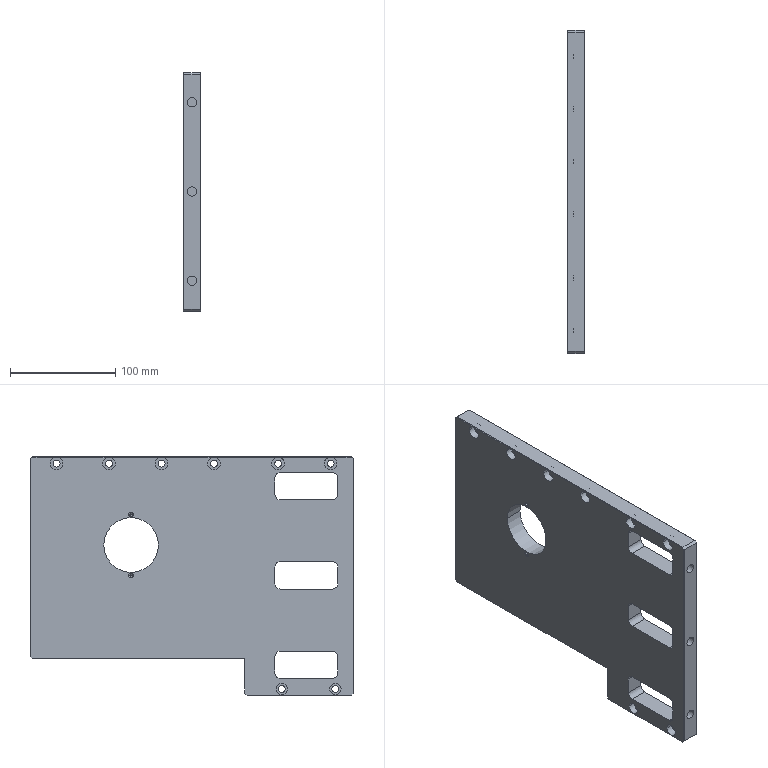Part | NX | 1 solid | 121 faces | box 17 x 308 x 227 mm | volume 940098 mm3 | cylinder 62 | plane 39 | cone 20 | commonest cylinder face diameters 6.6 x16 10 x12 12 x12 3.3 x10 9 x6 11 x4